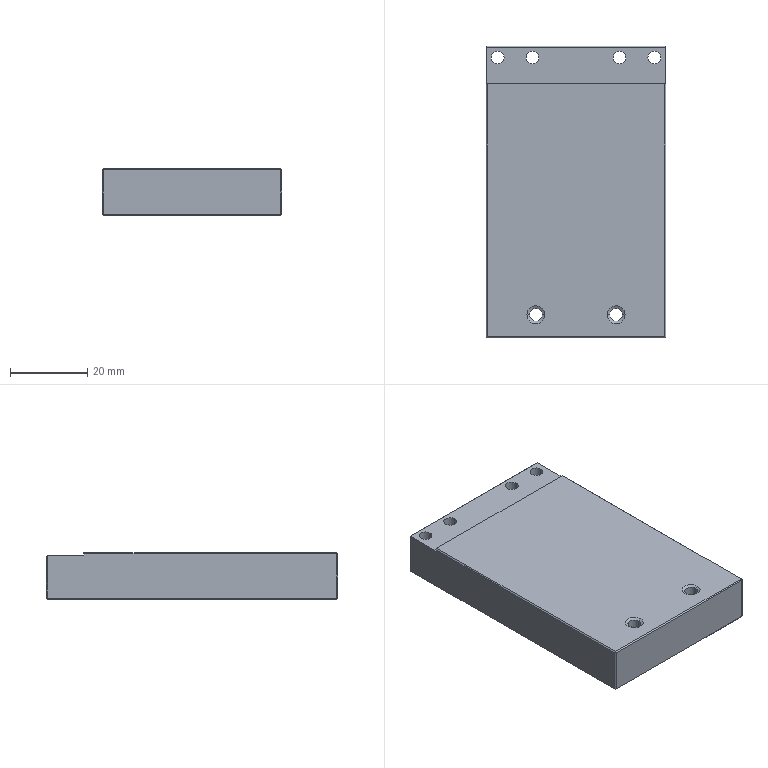Part | NX | 1 solid | 44 faces | box 46.5 x 75.4 x 12 mm | volume 41106 mm3 | plane 20 | cylinder 12 | cone 12 | commonest cylinder face diameters 3.3 x12
STEP:
#1=CARTESIAN_POINT('',(-134.2,260.1,-43.777));
#2=VERTEX_POINT('',#1);
#3=CARTESIAN_POINT('',(-88.3,260.1,-43.777));
#4=VERTEX_POINT('',#3);
#5=CARTESIAN_POINT('',(-111.25,260.1,-43.777));
#6=DIRECTION('',(1.,0.,0.));
#7=VECTOR('',#6,1000.);
#8=LINE('',#5,#7);
#9=EDGE_CURVE('',#2,#4,#8,.T.);
#10=ORIENTED_EDGE('',*,*,#9,.F.);
#11=CARTESIAN_POINT('',(-134.2,260.1,-33.14));
#12=VERTEX_POINT('',#11);
#13=CARTESIAN_POINT('',(-134.2,260.1,-38.458));
#14=DIRECTION('',(0.,0.,-1.));
#15=VECTOR('',#14,1000.);
#16=LINE('',#13,#15);
#17=EDGE_CURVE('',#12,#2,#16,.T.);
#18=ORIENTED_EDGE('',*,*,#17,.F.);
#19=CARTESIAN_POINT('',(-88.3,260.1,-33.14));
#20=VERTEX_POINT('',#19);
#21=CARTESIAN_POINT('',(-111.25,260.1,-33.14));
#22=DIRECTION('',(-1.,0.,0.));
#23=VECTOR('',#22,1000.);
#24=LINE('',#21,#23);
#25=EDGE_CURVE('',#20,#12,#24,.T.);
#26=ORIENTED_EDGE('',*,*,#25,.F.);
#27=CARTESIAN_POINT('',(-88.3,260.1,-38.458));
#28=DIRECTION('',(0.,0.,1.));
#29=VECTOR('',#28,1000.);
#30=LINE('',#27,#29);
#31=EDGE_CURVE('',#4,#20,#30,.T.);
#32=ORIENTED_EDGE('',*,*,#31,.F.);
#33=EDGE_LOOP('',(#10,#18,#26,#32));
#34=FACE_BOUND('',#33,.T.);
#35=CARTESIAN_POINT('',(-128.319,260.1,-42.779));
#36=DIRECTION('',(0.,1.,0.));
#37=DIRECTION('',(1.,0.,0.));
#38=AXIS2_PLACEMENT_3D('',#35,#36,#37);
#39=PLANE('',#38);
#40=ADVANCED_FACE('',(#34),#39,.T.);
#41=ORIENTED_EDGE('',*,*,#9,.T.);
#42=CARTESIAN_POINT('',(-88.15,259.95,-43.927));
#43=VERTEX_POINT('',#42);
#44=CARTESIAN_POINT('',(0.,171.8,-132.077));
#45=DIRECTION('',(0.5774,-0.5774,-0.5774));
#46=VECTOR('',#45,1000.);
#47=LINE('',#44,#46);
#48=EDGE_CURVE('',#4,#43,#47,.T.);
#49=ORIENTED_EDGE('',*,*,#48,.T.);
#50=CARTESIAN_POINT('',(-88.3,259.8,-44.077));
#51=VERTEX_POINT('',#50);
#52=CARTESIAN_POINT('',(0.,348.1,44.223));
#53=DIRECTION('',(-0.5774,-0.5774,-0.5774));
#54=VECTOR('',#53,1000.);
#55=LINE('',#52,#54);
#56=EDGE_CURVE('',#43,#51,#55,.T.);
#57=ORIENTED_EDGE('',*,*,#56,.T.);
#58=CARTESIAN_POINT('',(-134.2,259.8,-44.077));
#59=VERTEX_POINT('',#58);
#60=CARTESIAN_POINT('',(-111.25,259.8,-44.077));
#61=DIRECTION('',(1.,0.,0.));
#62=VECTOR('',#61,1000.);
#63=LINE('',#60,#62);
#64=EDGE_CURVE('',#59,#51,#63,.T.);
#65=ORIENTED_EDGE('',*,*,#64,.F.);
#66=CARTESIAN_POINT('',(-134.35,259.95,-43.927));
#67=VERTEX_POINT('',#66);
#68=CARTESIAN_POINT('',(125.6,0.,-303.877));
#69=DIRECTION('',(-0.5774,0.5774,0.5774));
#70=VECTOR('',#69,1000.);
#71=LINE('',#68,#70);
#72=EDGE_CURVE('',#59,#67,#71,.T.);
#73=ORIENTED_EDGE('',*,*,#72,.T.);
#74=CARTESIAN_POINT('',(0.,394.3,90.423));
#75=DIRECTION('',(-0.5774,-0.5774,-0.5774));
#76=VECTOR('',#75,1000.);
#77=LINE('',#74,#76);
#78=EDGE_CURVE('',#2,#67,#77,.T.);
#79=ORIENTED_EDGE('',*,*,#78,.F.);
#80=EDGE_LOOP('',(#41,#49,#57,#65,#73,#79));
#81=FACE_BOUND('',#80,.T.);
#82=CARTESIAN_POINT('',(-111.25,259.95,-43.927));
#83=DIRECTION('',(0.,-0.7071,0.7071));
#84=DIRECTION('',(-1.,0.,0.));
#85=AXIS2_PLACEMENT_3D('',#82,#83,#84);
#86=PLANE('',#85);
#87=ADVANCED_FACE('',(#81),#86,.F.);
#88=CARTESIAN_POINT('',(-134.5,185.,-32.377));
#89=VERTEX_POINT('',#88);
#90=CARTESIAN_POINT('',(-134.5,185.,-43.777));
#91=VERTEX_POINT('',#90);
#92=CARTESIAN_POINT('',(-134.5,185.,-37.927));
#93=DIRECTION('',(0.,0.,-1.));
#94=VECTOR('',#93,1000.);
#95=LINE('',#92,#94);
#96=EDGE_CURVE('',#89,#91,#95,.T.);
#97=ORIENTED_EDGE('',*,*,#96,.F.);
#98=CARTESIAN_POINT('',(-134.5,250.35,-32.377));
#99=VERTEX_POINT('',#98);
#100=CARTESIAN_POINT('',(-134.5,217.525,-32.377));
#101=DIRECTION('',(0.,1.,0.));
#102=VECTOR('',#101,1000.);
#103=LINE('',#100,#102);
#104=EDGE_CURVE('',#89,#99,#103,.T.);
#105=ORIENTED_EDGE('',*,*,#104,.T.);
#106=CARTESIAN_POINT('',(-134.5,250.35,-32.84));
#107=VERTEX_POINT('',#106);
#108=CARTESIAN_POINT('',(-134.5,250.35,0.));
#109=DIRECTION('',(0.,0.,1.));
#110=VECTOR('',#109,1000.);
#111=LINE('',#108,#110);
#112=EDGE_CURVE('',#107,#99,#111,.T.);
#113=ORIENTED_EDGE('',*,*,#112,.F.);
#114=CARTESIAN_POINT('',(-134.5,259.8,-32.84));
#115=VERTEX_POINT('',#114);
#116=CARTESIAN_POINT('',(-134.5,0.,-32.84));
#117=DIRECTION('',(0.,-1.,0.));
#118=VECTOR('',#117,1000.);
#119=LINE('',#116,#118);
#120=EDGE_CURVE('',#115,#107,#119,.T.);
#121=ORIENTED_EDGE('',*,*,#120,.F.);
#122=CARTESIAN_POINT('',(-134.5,259.8,-43.777));
#123=VERTEX_POINT('',#122);
#124=CARTESIAN_POINT('',(-134.5,259.8,-38.458));
#125=DIRECTION('',(0.,0.,-1.));
#126=VECTOR('',#125,1000.);
#127=LINE('',#124,#126);
#128=EDGE_CURVE('',#115,#123,#127,.T.);
#129=ORIENTED_EDGE('',*,*,#128,.T.);
#130=CARTESIAN_POINT('',(-134.5,222.55,-43.777));
#131=DIRECTION('',(0.,1.,0.));
#132=VECTOR('',#131,1000.);
#133=LINE('',#130,#132);
#134=EDGE_CURVE('',#91,#123,#133,.T.);
#135=ORIENTED_EDGE('',*,*,#134,.F.);
#136=EDGE_LOOP('',(#97,#105,#113,#121,#129,#135));
#137=FACE_BOUND('',#136,.T.);
#138=CARTESIAN_POINT('',(-134.5,208.7,-44.077));
#139=DIRECTION('',(-1.,0.,0.));
#140=DIRECTION('',(0.,0.,1.));
#141=AXIS2_PLACEMENT_3D('',#138,#139,#140);
#142=PLANE('',#141);
#143=ADVANCED_FACE('',(#137),#142,.T.);
#144=ORIENTED_EDGE('',*,*,#128,.F.);
#145=CARTESIAN_POINT('',(0.,394.3,-167.34));
#146=DIRECTION('',(-0.5774,-0.5774,0.5774));
#147=VECTOR('',#146,1000.);
#148=LINE('',#145,#147);
#149=EDGE_CURVE('',#12,#115,#148,.T.);
#150=ORIENTED_EDGE('',*,*,#149,.F.);
#151=ORIENTED_EDGE('',*,*,#17,.T.);
#152=ORIENTED_EDGE('',*,*,#78,.T.);
#153=CARTESIAN_POINT('',(-178.277,216.023,0.));
#154=DIRECTION('',(0.5774,0.5774,-0.5774));
#155=VECTOR('',#154,1000.);
#156=LINE('',#153,#155);
#157=EDGE_CURVE('',#123,#67,#156,.T.);
#158=ORIENTED_EDGE('',*,*,#157,.F.);
#159=EDGE_LOOP('',(#144,#150,#151,#152,#158));
#160=FACE_BOUND('',#159,.T.);
#161=CARTESIAN_POINT('',(-134.35,259.95,-38.458));
#162=DIRECTION('',(-0.7071,0.7071,0.));
#163=DIRECTION('',(0.,0.,1.));
#164=AXIS2_PLACEMENT_3D('',#161,#162,#163);
#165=PLANE('',#164);
#166=ADVANCED_FACE('',(#160),#165,.T.);
#167=ORIENTED_EDGE('',*,*,#134,.T.);
#168=ORIENTED_EDGE('',*,*,#157,.T.);
#169=ORIENTED_EDGE('',*,*,#72,.F.);
#170=CARTESIAN_POINT('',(-134.2,185.,-44.077));
#171=VERTEX_POINT('',#170);
#172=CARTESIAN_POINT('',(-134.2,222.55,-44.077));
#173=DIRECTION('',(0.,1.,0.));
#174=VECTOR('',#173,1000.);
#175=LINE('',#172,#174);
#176=EDGE_CURVE('',#171,#59,#175,.T.);
#177=ORIENTED_EDGE('',*,*,#176,.F.);
#178=CARTESIAN_POINT('',(-134.35,184.85,-43.927));
#179=VERTEX_POINT('',#178);
#180=CARTESIAN_POINT('',(-178.277,140.923,0.));
#181=DIRECTION('',(-0.5774,-0.5774,0.5774));
#182=VECTOR('',#181,1000.);
#183=LINE('',#180,#182);
#184=EDGE_CURVE('',#171,#179,#183,.T.);
#185=ORIENTED_EDGE('',*,*,#184,.T.);
#186=CARTESIAN_POINT('',(-178.277,228.777,0.));
#187=DIRECTION('',(0.5774,-0.5774,-0.5774));
#188=VECTOR('',#187,1000.);
#189=LINE('',#186,#188);
#190=EDGE_CURVE('',#91,#179,#189,.T.);
#191=ORIENTED_EDGE('',*,*,#190,.F.);
#192=EDGE_LOOP('',(#167,#168,#169,#177,#185,#191));
#193=FACE_BOUND('',#192,.T.);
#194=CARTESIAN_POINT('',(-134.35,222.55,-43.927));
#195=DIRECTION('',(0.7071,0.,0.7071));
#196=DIRECTION('',(0.,-1.,0.));
#197=AXIS2_PLACEMENT_3D('',#194,#195,#196);
#198=PLANE('',#197);
#199=ADVANCED_FACE('',(#193),#198,.F.);
#200=ORIENTED_EDGE('',*,*,#104,.F.);
#201=CARTESIAN_POINT('',(-134.35,184.85,-32.227));
#202=VERTEX_POINT('',#201);
#203=CARTESIAN_POINT('',(0.,50.5,102.123));
#204=DIRECTION('',(-0.5774,0.5774,-0.5774));
#205=VECTOR('',#204,1000.);
#206=LINE('',#203,#205);
#207=EDGE_CURVE('',#202,#89,#206,.T.);
#208=ORIENTED_EDGE('',*,*,#207,.F.);
#209=CARTESIAN_POINT('',(-134.2,185.,-32.077));
#210=VERTEX_POINT('',#209);
#211=CARTESIAN_POINT('',(0.,319.2,102.123));
#212=DIRECTION('',(-0.5774,-0.5774,-0.5774));
#213=VECTOR('',#212,1000.);
#214=LINE('',#211,#213);
#215=EDGE_CURVE('',#210,#202,#214,.T.);
#216=ORIENTED_EDGE('',*,*,#215,.F.);
#217=CARTESIAN_POINT('',(-134.2,250.35,-32.077));
#218=VERTEX_POINT('',#217);
#219=CARTESIAN_POINT('',(-134.2,217.525,-32.077));
#220=DIRECTION('',(0.,1.,0.));
#221=VECTOR('',#220,1000.);
#222=LINE('',#219,#221);
#223=EDGE_CURVE('',#210,#218,#222,.T.);
#224=ORIENTED_EDGE('',*,*,#223,.T.);
#225=CARTESIAN_POINT('',(0.,250.35,102.123));
#226=DIRECTION('',(0.7071,0.,0.7071));
#227=VECTOR('',#226,1000.);
#228=LINE('',#225,#227);
#229=EDGE_CURVE('',#99,#218,#228,.T.);
#230=ORIENTED_EDGE('',*,*,#229,.F.);
#231=EDGE_LOOP('',(#200,#208,#216,#224,#230));
#232=FACE_BOUND('',#231,.T.);
#233=CARTESIAN_POINT('',(-134.35,217.525,-32.227));
#234=DIRECTION('',(-0.7071,0.,0.7071));
#235=DIRECTION('',(0.,1.,0.));
#236=AXIS2_PLACEMENT_3D('',#233,#234,#235);
#237=PLANE('',#236);
#238=ADVANCED_FACE('',(#232),#237,.T.);
#239=ORIENTED_EDGE('',*,*,#96,.T.);
#240=ORIENTED_EDGE('',*,*,#190,.T.);
#241=CARTESIAN_POINT('',(-134.2,184.7,-43.777));
#242=VERTEX_POINT('',#241);
#243=CARTESIAN_POINT('',(50.5,0.,140.923));
#244=DIRECTION('',(0.5774,-0.5774,0.5774));
#245=VECTOR('',#244,1000.);
#246=LINE('',#243,#245);
#247=EDGE_CURVE('',#179,#242,#246,.T.);
#248=ORIENTED_EDGE('',*,*,#247,.T.);
#249=CARTESIAN_POINT('',(-134.2,184.7,-32.377));
#250=VERTEX_POINT('',#249);
#251=CARTESIAN_POINT('',(-134.2,184.7,-37.927));
#252=DIRECTION('',(0.,0.,-1.));
#253=VECTOR('',#252,1000.);
#254=LINE('',#251,#253);
#255=EDGE_CURVE('',#250,#242,#254,.T.);
#256=ORIENTED_EDGE('',*,*,#255,.F.);
#257=CARTESIAN_POINT('',(50.5,0.,-217.077));
#258=DIRECTION('',(-0.5774,0.5774,0.5774));
#259=VECTOR('',#258,1000.);
#260=LINE('',#257,#259);
#261=EDGE_CURVE('',#250,#202,#260,.T.);
#262=ORIENTED_EDGE('',*,*,#261,.T.);
#263=ORIENTED_EDGE('',*,*,#207,.T.);
#264=EDGE_LOOP('',(#239,#240,#248,#256,#262,#263));
#265=FACE_BOUND('',#264,.T.);
#266=CARTESIAN_POINT('',(-134.35,184.85,-37.927));
#267=DIRECTION('',(0.7071,0.7071,0.));
#268=DIRECTION('',(0.,0.,-1.));
#269=AXIS2_PLACEMENT_3D('',#266,#267,#268);
#270=PLANE('',#269);
#271=ADVANCED_FACE('',(#265),#270,.F.);
#272=CARTESIAN_POINT('',(-88.,259.8,-43.777));
#273=VERTEX_POINT('',#272);
#274=CARTESIAN_POINT('',(-88.,259.8,-32.84));
#275=VERTEX_POINT('',#274);
#276=CARTESIAN_POINT('',(-88.,259.8,-38.458));
#277=DIRECTION('',(0.,0.,1.));
#278=VECTOR('',#277,1000.);
#279=LINE('',#276,#278);
#280=EDGE_CURVE('',#273,#275,#279,.T.);
#281=ORIENTED_EDGE('',*,*,#280,.T.);
#282=CARTESIAN_POINT('',(-88.,250.35,-32.84));
#283=VERTEX_POINT('',#282);
#284=CARTESIAN_POINT('',(-88.,0.,-32.84));
#285=DIRECTION('',(0.,1.,0.));
#286=VECTOR('',#285,1000.);
#287=LINE('',#284,#286);
#288=EDGE_CURVE('',#283,#275,#287,.T.);
#289=ORIENTED_EDGE('',*,*,#288,.F.);
#290=CARTESIAN_POINT('',(-88.,250.35,-32.377));
#291=VERTEX_POINT('',#290);
#292=CARTESIAN_POINT('',(-88.,250.35,0.));
#293=DIRECTION('',(0.,0.,-1.));
#294=VECTOR('',#293,1000.);
#295=LINE('',#292,#294);
#296=EDGE_CURVE('',#291,#283,#295,.T.);
#297=ORIENTED_EDGE('',*,*,#296,.F.);
#298=CARTESIAN_POINT('',(-88.,185.,-32.377));
#299=VERTEX_POINT('',#298);
#300=CARTESIAN_POINT('',(-88.,217.525,-32.377));
#301=DIRECTION('',(0.,1.,0.));
#302=VECTOR('',#301,1000.);
#303=LINE('',#300,#302);
#304=EDGE_CURVE('',#299,#291,#303,.T.);
#305=ORIENTED_EDGE('',*,*,#304,.F.);
#306=CARTESIAN_POINT('',(-88.,185.,-43.777));
#307=VERTEX_POINT('',#306);
#308=CARTESIAN_POINT('',(-88.,185.,-37.927));
#309=DIRECTION('',(0.,0.,1.));
#310=VECTOR('',#309,1000.);
#311=LINE('',#308,#310);
#312=EDGE_CURVE('',#307,#299,#311,.T.);
#313=ORIENTED_EDGE('',*,*,#312,.F.);
#314=CARTESIAN_POINT('',(-88.,222.55,-43.777));
#315=DIRECTION('',(0.,1.,0.));
#316=VECTOR('',#315,1000.);
#317=LINE('',#314,#316);
#318=EDGE_CURVE('',#307,#273,#317,.T.);
#319=ORIENTED_EDGE('',*,*,#318,.T.);
#320=EDGE_LOOP('',(#281,#289,#297,#305,#313,#319));
#321=FACE_BOUND('',#320,.T.);
#322=CARTESIAN_POINT('',(-88.,208.7,-40.863));
#323=DIRECTION('',(1.,0.,0.));
#324=DIRECTION('',(0.,-1.,0.));
#325=AXIS2_PLACEMENT_3D('',#322,#323,#324);
#326=PLANE('',#325);
#327=ADVANCED_FACE('',(#321),#326,.T.);
#328=ORIENTED_EDGE('',*,*,#312,.T.);
#329=CARTESIAN_POINT('',(-88.15,184.85,-32.227));
#330=VERTEX_POINT('',#329);
#331=CARTESIAN_POINT('',(-273.,0.,152.623));
#332=DIRECTION('',(-0.5774,-0.5774,0.5774));
#333=VECTOR('',#332,1000.);
#334=LINE('',#331,#333);
#335=EDGE_CURVE('',#299,#330,#334,.T.);
#336=ORIENTED_EDGE('',*,*,#335,.T.);
#337=CARTESIAN_POINT('',(-88.3,184.7,-32.377));
#338=VERTEX_POINT('',#337);
#339=CARTESIAN_POINT('',(-273.,0.,-217.077));
#340=DIRECTION('',(0.5774,0.5774,0.5774));
#341=VECTOR('',#340,1000.);
#342=LINE('',#339,#341);
#343=EDGE_CURVE('',#338,#330,#342,.T.);
#344=ORIENTED_EDGE('',*,*,#343,.F.);
#345=CARTESIAN_POINT('',(-88.3,184.7,-43.777));
#346=VERTEX_POINT('',#345);
#347=CARTESIAN_POINT('',(-88.3,184.7,-37.927));
#348=DIRECTION('',(0.,0.,1.));
#349=VECTOR('',#348,1000.);
#350=LINE('',#347,#349);
#351=EDGE_CURVE('',#346,#338,#350,.T.);
#352=ORIENTED_EDGE('',*,*,#351,.F.);
#353=CARTESIAN_POINT('',(-88.15,184.85,-43.927));
#354=VERTEX_POINT('',#353);
#355=CARTESIAN_POINT('',(-132.077,140.923,0.));
#356=DIRECTION('',(0.5774,0.5774,-0.5774));
#357=VECTOR('',#356,1000.);
#358=LINE('',#355,#357);
#359=EDGE_CURVE('',#346,#354,#358,.T.);
#360=ORIENTED_EDGE('',*,*,#359,.T.);
#361=CARTESIAN_POINT('',(0.,273.,44.223));
#362=DIRECTION('',(0.5774,0.5774,0.5774));
#363=VECTOR('',#362,1000.);
#364=LINE('',#361,#363);
#365=EDGE_CURVE('',#354,#307,#364,.T.);
#366=ORIENTED_EDGE('',*,*,#365,.T.);
#367=EDGE_LOOP('',(#328,#336,#344,#352,#360,#366));
#368=FACE_BOUND('',#367,.T.);
#369=CARTESIAN_POINT('',(-88.15,184.85,-37.927));
#370=DIRECTION('',(-0.7071,0.7071,0.));
#371=DIRECTION('',(0.,0.,1.));
#372=AXIS2_PLACEMENT_3D('',#369,#370,#371);
#373=PLANE('',#372);
#374=ADVANCED_FACE('',(#368),#373,.F.);
#375=ORIENTED_EDGE('',*,*,#304,.T.);
#376=CARTESIAN_POINT('',(-88.3,250.35,-32.077));
#377=VERTEX_POINT('',#376);
#378=CARTESIAN_POINT('',(-120.377,250.35,0.));
#379=DIRECTION('',(-0.7071,0.,0.7071));
#380=VECTOR('',#379,1000.);
#381=LINE('',#378,#380);
#382=EDGE_CURVE('',#291,#377,#381,.T.);
#383=ORIENTED_EDGE('',*,*,#382,.T.);
#384=CARTESIAN_POINT('',(-88.3,185.,-32.077));
#385=VERTEX_POINT('',#384);
#386=CARTESIAN_POINT('',(-88.3,217.525,-32.077));
#387=DIRECTION('',(0.,1.,0.));
#388=VECTOR('',#387,1000.);
#389=LINE('',#386,#388);
#390=EDGE_CURVE('',#385,#377,#389,.T.);
#391=ORIENTED_EDGE('',*,*,#390,.F.);
#392=CARTESIAN_POINT('',(96.7,0.,-217.077));
#393=DIRECTION('',(-0.5774,0.5774,0.5774));
#394=VECTOR('',#393,1000.);
#395=LINE('',#392,#394);
#396=EDGE_CURVE('',#330,#385,#395,.T.);
#397=ORIENTED_EDGE('',*,*,#396,.F.);
#398=ORIENTED_EDGE('',*,*,#335,.F.);
#399=EDGE_LOOP('',(#375,#383,#391,#397,#398));
#400=FACE_BOUND('',#399,.T.);
#401=CARTESIAN_POINT('',(-88.15,217.525,-32.227));
#402=DIRECTION('',(-0.7071,0.,-0.7071));
#403=DIRECTION('',(-0.7071,0.,0.7071));
#404=AXIS2_PLACEMENT_3D('',#401,#402,#403);
#405=PLANE('',#404);
#406=ADVANCED_FACE('',(#400),#405,.F.);
#407=ORIENTED_EDGE('',*,*,#318,.F.);
#408=ORIENTED_EDGE('',*,*,#365,.F.);
#409=CARTESIAN_POINT('',(-88.3,185.,-44.077));
#410=VERTEX_POINT('',#409);
#411=CARTESIAN_POINT('',(0.,96.7,44.223));
#412=DIRECTION('',(0.5774,-0.5774,0.5774));
#413=VECTOR('',#412,1000.);
#414=LINE('',#411,#413);
#415=EDGE_CURVE('',#410,#354,#414,.T.);
#416=ORIENTED_EDGE('',*,*,#415,.F.);
#417=CARTESIAN_POINT('',(-88.3,222.55,-44.077));
#418=DIRECTION('',(0.,1.,0.));
#419=VECTOR('',#418,1000.);
#420=LINE('',#417,#419);
#421=EDGE_CURVE('',#410,#51,#420,.T.);
#422=ORIENTED_EDGE('',*,*,#421,.T.);
#423=ORIENTED_EDGE('',*,*,#56,.F.);
#424=CARTESIAN_POINT('',(0.,171.8,44.223));
#425=DIRECTION('',(0.5774,-0.5774,0.5774));
#426=VECTOR('',#425,1000.);
#427=LINE('',#424,#426);
#428=EDGE_CURVE('',#43,#273,#427,.T.);
#429=ORIENTED_EDGE('',*,*,#428,.T.);
#430=EDGE_LOOP('',(#407,#408,#416,#422,#423,#429));
#431=FACE_BOUND('',#430,.T.);
#432=CARTESIAN_POINT('',(-88.15,222.55,-43.927));
#433=DIRECTION('',(0.7071,0.,-0.7071));
#434=DIRECTION('',(0.,-1.,0.));
#435=AXIS2_PLACEMENT_3D('',#432,#433,#434);
#436=PLANE('',#435);
#437=ADVANCED_FACE('',(#431),#436,.T.);
#438=ORIENTED_EDGE('',*,*,#280,.F.);
#439=ORIENTED_EDGE('',*,*,#428,.F.);
#440=ORIENTED_EDGE('',*,*,#48,.F.);
#441=ORIENTED_EDGE('',*,*,#31,.T.);
#442=CARTESIAN_POINT('',(0.,171.8,55.16));
#443=DIRECTION('',(0.5774,-0.5774,0.5774));
#444=VECTOR('',#443,1000.);
#445=LINE('',#442,#444);
#446=EDGE_CURVE('',#20,#275,#445,.T.);
#447=ORIENTED_EDGE('',*,*,#446,.T.);
#448=EDGE_LOOP('',(#438,#439,#440,#441,#447));
#449=FACE_BOUND('',#448,.T.);
#450=CARTESIAN_POINT('',(-88.15,259.95,-38.458));
#451=DIRECTION('',(0.7071,0.7071,0.));
#452=DIRECTION('',(0.,0.,-1.));
#453=AXIS2_PLACEMENT_3D('',#450,#451,#452);
#454=PLANE('',#453);
#455=ADVANCED_FACE('',(#449),#454,.T.);
#456=CARTESIAN_POINT('',(-132.,185.,-44.077));
#457=DIRECTION('',(-1.,0.,0.));
#458=VECTOR('',#457,1000.);
#459=LINE('',#456,#458);
#460=EDGE_CURVE('',#410,#171,#459,.T.);
#461=ORIENTED_EDGE('',*,*,#460,.F.);
#462=ORIENTED_EDGE('',*,*,#415,.T.);
#463=ORIENTED_EDGE('',*,*,#359,.F.);
#464=CARTESIAN_POINT('',(-132.,184.7,-43.777));
#465=DIRECTION('',(-1.,0.,0.));
#466=VECTOR('',#465,1000.);
#467=LINE('',#464,#466);
#468=EDGE_CURVE('',#346,#242,#467,.T.);
#469=ORIENTED_EDGE('',*,*,#468,.T.);
#470=ORIENTED_EDGE('',*,*,#247,.F.);
#471=ORIENTED_EDGE('',*,*,#184,.F.);
#472=EDGE_LOOP('',(#461,#462,#463,#469,#470,#471));
#473=FACE_BOUND('',#472,.T.);
#474=CARTESIAN_POINT('',(-111.25,184.85,-43.927));
#475=DIRECTION('',(0.,0.7071,0.7071));
#476=DIRECTION('',(1.,0.,0.));
#477=AXIS2_PLACEMENT_3D('',#474,#475,#476);
#478=PLANE('',#477);
#479=ADVANCED_FACE('',(#473),#478,.F.);
#480=CARTESIAN_POINT('',(-111.25,185.,-32.077));
#481=DIRECTION('',(-1.,0.,0.));
#482=VECTOR('',#481,1000.);
#483=LINE('',#480,#482);
#484=EDGE_CURVE('',#385,#210,#483,.T.);
#485=ORIENTED_EDGE('',*,*,#484,.F.);
#486=ORIENTED_EDGE('',*,*,#390,.T.);
#487=CARTESIAN_POINT('',(0.,250.35,-32.077));
#488=DIRECTION('',(1.,0.,0.));
#489=VECTOR('',#488,1000.);
#490=LINE('',#487,#489);
#491=EDGE_CURVE('',#218,#377,#490,.T.);
#492=ORIENTED_EDGE('',*,*,#491,.F.);
#493=ORIENTED_EDGE('',*,*,#223,.F.);
#494=EDGE_LOOP('',(#485,#486,#492,#493));
#495=FACE_BOUND('',#494,.T.);
#496=CARTESIAN_POINT('',(-103.19,190.7,-32.077));
#497=VERTEX_POINT('',#496);
#498=CARTESIAN_POINT('',(-98.56,190.7,-32.077));
#499=VERTEX_POINT('',#498);
#500=CARTESIAN_POINT('',(-100.875,190.7,-32.077));
#501=DIRECTION('',(0.,0.,1.));
#502=DIRECTION('',(1.,0.,0.));
#503=AXIS2_PLACEMENT_3D('',#500,#501,#502);
#504=CIRCLE('',#503,2.315);
#505=EDGE_CURVE('',#497,#499,#504,.T.);
#506=ORIENTED_EDGE('',*,*,#505,.F.);
#507=CARTESIAN_POINT('',(-100.875,190.7,-32.077));
#508=DIRECTION('',(0.,0.,1.));
#509=DIRECTION('',(1.,0.,0.));
#510=AXIS2_PLACEMENT_3D('',#507,#508,#509);
#511=CIRCLE('',#510,2.315);
#512=EDGE_CURVE('',#499,#497,#511,.T.);
#513=ORIENTED_EDGE('',*,*,#512,.F.);
#514=EDGE_LOOP('',(#506,#513));
#515=FACE_BOUND('',#514,.T.);
#516=CARTESIAN_POINT('',(-123.94,190.7,-32.077));
#517=VERTEX_POINT('',#516);
#518=CARTESIAN_POINT('',(-119.31,190.7,-32.077));
#519=VERTEX_POINT('',#518);
#520=CARTESIAN_POINT('',(-121.625,190.7,-32.077));
#521=DIRECTION('',(0.,0.,1.));
#522=DIRECTION('',(1.,0.,0.));
#523=AXIS2_PLACEMENT_3D('',#520,#521,#522);
#524=CIRCLE('',#523,2.315);
#525=EDGE_CURVE('',#517,#519,#524,.T.);
#526=ORIENTED_EDGE('',*,*,#525,.F.);
#527=CARTESIAN_POINT('',(-121.625,190.7,-32.077));
#528=DIRECTION('',(0.,0.,1.));
#529=DIRECTION('',(1.,0.,0.));
#530=AXIS2_PLACEMENT_3D('',#527,#528,#529);
#531=CIRCLE('',#530,2.315);
#532=EDGE_CURVE('',#519,#517,#531,.T.);
#533=ORIENTED_EDGE('',*,*,#532,.F.);
#534=EDGE_LOOP('',(#526,#533));
#535=FACE_BOUND('',#534,.T.);
#536=CARTESIAN_POINT('',(-137.,208.7,-32.077));
#537=DIRECTION('',(0.,0.,1.));
#538=DIRECTION('',(1.,0.,0.));
#539=AXIS2_PLACEMENT_3D('',#536,#537,#538);
#540=PLANE('',#539);
#541=ADVANCED_FACE('',(#495,#515,#535),#540,.T.);
#542=CARTESIAN_POINT('',(-111.25,184.7,-32.377));
#543=DIRECTION('',(-1.,0.,0.));
#544=VECTOR('',#543,1000.);
#545=LINE('',#542,#544);
#546=EDGE_CURVE('',#338,#250,#545,.T.);
#547=ORIENTED_EDGE('',*,*,#546,.T.);
#548=ORIENTED_EDGE('',*,*,#255,.T.);
#549=ORIENTED_EDGE('',*,*,#468,.F.);
#550=ORIENTED_EDGE('',*,*,#351,.T.);
#551=EDGE_LOOP('',(#547,#548,#549,#550));
#552=FACE_BOUND('',#551,.T.);
#553=CARTESIAN_POINT('',(-128.319,184.7,-42.779));
#554=DIRECTION('',(0.,1.,0.));
#555=DIRECTION('',(1.,0.,0.));
#556=AXIS2_PLACEMENT_3D('',#553,#554,#555);
#557=PLANE('',#556);
#558=ADVANCED_FACE('',(#552),#557,.F.);
#559=CARTESIAN_POINT('',(-102.525,190.7,-32.461));
#560=VERTEX_POINT('',#559);
#561=CARTESIAN_POINT('',(-99.225,190.7,-32.461));
#562=VERTEX_POINT('',#561);
#563=CARTESIAN_POINT('',(-100.875,190.7,-32.461));
#564=DIRECTION('',(0.,0.,1.));
#565=DIRECTION('',(1.,0.,0.));
#566=AXIS2_PLACEMENT_3D('',#563,#564,#565);
#567=CIRCLE('',#566,1.65);
#568=EDGE_CURVE('',#560,#562,#567,.T.);
#569=ORIENTED_EDGE('',*,*,#568,.T.);
#570=CARTESIAN_POINT('',(-99.225,190.7,-44.077));
#571=VERTEX_POINT('',#570);
#572=CARTESIAN_POINT('',(-99.225,190.7,-36.077));
#573=DIRECTION('',(0.,0.,1.));
#574=VECTOR('',#573,1000.);
#575=LINE('',#572,#574);
#576=EDGE_CURVE('',#571,#562,#575,.T.);
#577=ORIENTED_EDGE('',*,*,#576,.F.);
#578=CARTESIAN_POINT('',(-102.525,190.7,-44.077));
#579=VERTEX_POINT('',#578);
#580=CARTESIAN_POINT('',(-100.875,190.7,-44.077));
#581=DIRECTION('',(0.,0.,1.));
#582=DIRECTION('',(1.,0.,0.));
#583=AXIS2_PLACEMENT_3D('',#580,#581,#582);
#584=CIRCLE('',#583,1.65);
#585=EDGE_CURVE('',#579,#571,#584,.T.);
#586=ORIENTED_EDGE('',*,*,#585,.F.);
#587=CARTESIAN_POINT('',(-102.525,190.7,-36.077));
#588=DIRECTION('',(0.,0.,1.));
#589=VECTOR('',#588,1000.);
#590=LINE('',#587,#589);
#591=EDGE_CURVE('',#579,#560,#590,.T.);
#592=ORIENTED_EDGE('',*,*,#591,.T.);
#593=EDGE_LOOP('',(#569,#577,#586,#592));
#594=FACE_BOUND('',#593,.T.);
#595=CARTESIAN_POINT('',(-100.875,190.7,-36.077));
#596=DIRECTION('',(0.,0.,1.));
#597=DIRECTION('',(1.,0.,0.));
#598=AXIS2_PLACEMENT_3D('',#595,#596,#597);
#599=CYLINDRICAL_SURFACE('',#598,1.65);
#600=ADVANCED_FACE('',(#594),#599,.F.);
#601=CARTESIAN_POINT('',(-89.35,257.1,-43.693));
#602=VERTEX_POINT('',#601);
#603=CARTESIAN_POINT('',(-92.65,257.1,-43.693));
#604=VERTEX_POINT('',#603);
#605=CARTESIAN_POINT('',(-91.,257.1,-43.693));
#606=DIRECTION('',(0.,0.,-1.));
#607=DIRECTION('',(-1.,0.,0.));
#608=AXIS2_PLACEMENT_3D('',#605,#606,#607);
#609=CIRCLE('',#608,1.65);
#610=EDGE_CURVE('',#602,#604,#609,.T.);
#611=ORIENTED_EDGE('',*,*,#610,.F.);
#612=CARTESIAN_POINT('',(-88.685,257.1,-44.077));
#613=VERTEX_POINT('',#612);
#614=CARTESIAN_POINT('',(-89.35,257.1,-43.693));
#615=DIRECTION('',(0.866,0.,-0.5));
#616=VECTOR('',#615,1000.);
#617=LINE('',#614,#616);
#618=EDGE_CURVE('',#613,#602,#617,.F.);
#619=ORIENTED_EDGE('',*,*,#618,.F.);
#620=CARTESIAN_POINT('',(-93.315,257.1,-44.077));
#621=VERTEX_POINT('',#620);
#622=CARTESIAN_POINT('',(-91.,257.1,-44.077));
#623=DIRECTION('',(0.,0.,-1.));
#624=DIRECTION('',(-1.,0.,0.));
#625=AXIS2_PLACEMENT_3D('',#622,#623,#624);
#626=CIRCLE('',#625,2.315);
#627=EDGE_CURVE('',#613,#621,#626,.T.);
#628=ORIENTED_EDGE('',*,*,#627,.T.);
#629=CARTESIAN_POINT('',(-92.65,257.1,-43.693));
#630=DIRECTION('',(-0.866,0.,-0.5));
#631=VECTOR('',#630,1000.);
#632=LINE('',#629,#631);
#633=EDGE_CURVE('',#621,#604,#632,.F.);
#634=ORIENTED_EDGE('',*,*,#633,.T.);
#635=EDGE_LOOP('',(#611,#619,#628,#634));
#636=FACE_BOUND('',#635,.T.);
#637=CARTESIAN_POINT('',(-91.,257.1,-43.693));
#638=DIRECTION('',(0.,0.,-1.));
#639=DIRECTION('',(-1.,0.,0.));
#640=AXIS2_PLACEMENT_3D('',#637,#638,#639);
#641=CONICAL_SURFACE('',#640,1.65,1.047);
#642=ADVANCED_FACE('',(#636),#641,.F.);
#643=ORIENTED_EDGE('',*,*,#460,.T.);
#644=ORIENTED_EDGE('',*,*,#176,.T.);
#645=ORIENTED_EDGE('',*,*,#64,.T.);
#646=ORIENTED_EDGE('',*,*,#421,.F.);
#647=EDGE_LOOP('',(#643,#644,#645,#646));
#648=FACE_BOUND('',#647,.T.);
#649=CARTESIAN_POINT('',(-97.685,257.1,-44.077));
#650=VERTEX_POINT('',#649);
#651=CARTESIAN_POINT('',(-102.315,257.1,-44.077));
#652=VERTEX_POINT('',#651);
#653=CARTESIAN_POINT('',(-100.,257.1,-44.077));
#654=DIRECTION('',(0.,0.,-1.));
#655=DIRECTION('',(-1.,0.,0.));
#656=AXIS2_PLACEMENT_3D('',#653,#654,#655);
#657=CIRCLE('',#656,2.315);
#658=EDGE_CURVE('',#650,#652,#657,.T.);
#659=ORIENTED_EDGE('',*,*,#658,.F.);
#660=CARTESIAN_POINT('',(-100.,257.1,-44.077));
#661=DIRECTION('',(0.,0.,-1.));
#662=DIRECTION('',(-1.,0.,0.));
#663=AXIS2_PLACEMENT_3D('',#660,#661,#662);
#664=CIRCLE('',#663,2.315);
#665=EDGE_CURVE('',#652,#650,#664,.T.);
#666=ORIENTED_EDGE('',*,*,#665,.F.);
#667=EDGE_LOOP('',(#659,#666));
#668=FACE_BOUND('',#667,.T.);
#669=CARTESIAN_POINT('',(-129.185,257.1,-44.077));
#670=VERTEX_POINT('',#669);
#671=CARTESIAN_POINT('',(-133.815,257.1,-44.077));
#672=VERTEX_POINT('',#671);
#673=CARTESIAN_POINT('',(-131.5,257.1,-44.077));
#674=DIRECTION('',(0.,0.,-1.));
#675=DIRECTION('',(-1.,0.,0.));
#676=AXIS2_PLACEMENT_3D('',#673,#674,#675);
#677=CIRCLE('',#676,2.315);
#678=EDGE_CURVE('',#670,#672,#677,.T.);
#679=ORIENTED_EDGE('',*,*,#678,.F.);
#680=CARTESIAN_POINT('',(-131.5,257.1,-44.077));
#681=DIRECTION('',(0.,0.,-1.));
#682=DIRECTION('',(-1.,0.,0.));
#683=AXIS2_PLACEMENT_3D('',#680,#681,#682);
#684=CIRCLE('',#683,2.315);
#685=EDGE_CURVE('',#672,#670,#684,.T.);
#686=ORIENTED_EDGE('',*,*,#685,.F.);
#687=EDGE_LOOP('',(#679,#686));
#688=FACE_BOUND('',#687,.T.);
#689=ORIENTED_EDGE('',*,*,#627,.F.);
#690=CARTESIAN_POINT('',(-91.,257.1,-44.077));
#691=DIRECTION('',(0.,0.,-1.));
#692=DIRECTION('',(-1.,0.,0.));
#693=AXIS2_PLACEMENT_3D('',#690,#691,#692);
#694=CIRCLE('',#693,2.315);
#695=EDGE_CURVE('',#621,#613,#694,.T.);
#696=ORIENTED_EDGE('',*,*,#695,.F.);
#697=EDGE_LOOP('',(#689,#696));
#698=FACE_BOUND('',#697,.T.);
#699=CARTESIAN_POINT('',(-123.275,190.7,-44.077));
#700=VERTEX_POINT('',#699);
#701=CARTESIAN_POINT('',(-119.975,190.7,-44.077));
#702=VERTEX_POINT('',#701);
#703=CARTESIAN_POINT('',(-121.625,190.7,-44.077));
#704=DIRECTION('',(0.,0.,1.));
#705=DIRECTION('',(1.,0.,0.));
#706=AXIS2_PLACEMENT_3D('',#703,#704,#705);
#707=CIRCLE('',#706,1.65);
#708=EDGE_CURVE('',#700,#702,#707,.T.);
#709=ORIENTED_EDGE('',*,*,#708,.T.);
#710=CARTESIAN_POINT('',(-121.625,190.7,-44.077));
#711=DIRECTION('',(0.,0.,1.));
#712=DIRECTION('',(1.,0.,0.));
#713=AXIS2_PLACEMENT_3D('',#710,#711,#712);
#714=CIRCLE('',#713,1.65);
#715=EDGE_CURVE('',#702,#700,#714,.T.);
#716=ORIENTED_EDGE('',*,*,#715,.T.);
#717=EDGE_LOOP('',(#709,#716));
#718=FACE_BOUND('',#717,.T.);
#719=CARTESIAN_POINT('',(-120.185,257.1,-44.077));
#720=VERTEX_POINT('',#719);
#721=CARTESIAN_POINT('',(-124.815,257.1,-44.077));
#722=VERTEX_POINT('',#721);
#723=CARTESIAN_POINT('',(-122.5,257.1,-44.077));
#724=DIRECTION('',(0.,0.,-1.));
#725=DIRECTION('',(-1.,0.,0.));
#726=AXIS2_PLACEMENT_3D('',#723,#724,#725);
#727=CIRCLE('',#726,2.315);
#728=EDGE_CURVE('',#720,#722,#727,.T.);
#729=ORIENTED_EDGE('',*,*,#728,.F.);
#730=CARTESIAN_POINT('',(-122.5,257.1,-44.077));
#731=DIRECTION('',(0.,0.,-1.));
#732=DIRECTION('',(-1.,0.,0.));
#733=AXIS2_PLACEMENT_3D('',#730,#731,#732);
#734=CIRCLE('',#733,2.315);
#735=EDGE_CURVE('',#722,#720,#734,.T.);
#736=ORIENTED_EDGE('',*,*,#735,.F.);
#737=EDGE_LOOP('',(#729,#736));
#738=FACE_BOUND('',#737,.T.);
#739=ORIENTED_EDGE('',*,*,#585,.T.);
#740=CARTESIAN_POINT('',(-100.875,190.7,-44.077));
#741=DIRECTION('',(0.,0.,1.));
#742=DIRECTION('',(1.,0.,0.));
#743=AXIS2_PLACEMENT_3D('',#740,#741,#742);
#744=CIRCLE('',#743,1.65);
#745=EDGE_CURVE('',#571,#579,#744,.T.);
#746=ORIENTED_EDGE('',*,*,#745,.T.);
#747=EDGE_LOOP('',(#739,#746));
#748=FACE_BOUND('',#747,.T.);
#749=CARTESIAN_POINT('',(-88.698,210.445,-44.077));
#750=DIRECTION('',(0.,0.,-1.));
#751=DIRECTION('',(0.,-1.,0.));
#752=AXIS2_PLACEMENT_3D('',#749,#750,#751);
#753=PLANE('',#752);
#754=ADVANCED_FACE('',(#648,#668,#688,#698,#718,#738,#748),#753,.T.);
#755=CARTESIAN_POINT('',(-123.275,190.7,-32.461));
#756=VERTEX_POINT('',#755);
#757=CARTESIAN_POINT('',(-119.975,190.7,-32.461));
#758=VERTEX_POINT('',#757);
#759=CARTESIAN_POINT('',(-121.625,190.7,-32.461));
#760=DIRECTION('',(0.,0.,1.));
#761=DIRECTION('',(1.,0.,0.));
#762=AXIS2_PLACEMENT_3D('',#759,#760,#761);
#763=CIRCLE('',#762,1.65);
#764=EDGE_CURVE('',#756,#758,#763,.T.);
#765=ORIENTED_EDGE('',*,*,#764,.T.);
#766=CARTESIAN_POINT('',(-119.975,190.7,-36.077));
#767=DIRECTION('',(0.,0.,1.));
#768=VECTOR('',#767,1000.);
#769=LINE('',#766,#768);
#770=EDGE_CURVE('',#702,#758,#769,.T.);
#771=ORIENTED_EDGE('',*,*,#770,.F.);
#772=ORIENTED_EDGE('',*,*,#708,.F.);
#773=CARTESIAN_POINT('',(-123.275,190.7,-36.077));
#774=DIRECTION('',(0.,0.,1.));
#775=VECTOR('',#774,1000.);
#776=LINE('',#773,#775);
#777=EDGE_CURVE('',#700,#756,#776,.T.);
#778=ORIENTED_EDGE('',*,*,#777,.T.);
#779=EDGE_LOOP('',(#765,#771,#772,#778));
#780=FACE_BOUND('',#779,.T.);
#781=CARTESIAN_POINT('',(-121.625,190.7,-36.077));
#782=DIRECTION('',(0.,0.,1.));
#783=DIRECTION('',(1.,0.,0.));
#784=AXIS2_PLACEMENT_3D('',#781,#782,#783);
#785=CYLINDRICAL_SURFACE('',#784,1.65);
#786=ADVANCED_FACE('',(#780),#785,.F.);
#787=ORIENTED_EDGE('',*,*,#764,.F.);
#788=CARTESIAN_POINT('',(-123.275,190.7,-32.461));
#789=DIRECTION('',(-0.866,0.,0.5));
#790=VECTOR('',#789,1000.);
#791=LINE('',#788,#790);
#792=EDGE_CURVE('',#756,#517,#791,.T.);
#793=ORIENTED_EDGE('',*,*,#792,.T.);
#794=ORIENTED_EDGE('',*,*,#525,.T.);
#795=CARTESIAN_POINT('',(-119.975,190.7,-32.461));
#796=DIRECTION('',(0.866,0.,0.5));
#797=VECTOR('',#796,1000.);
#798=LINE('',#795,#797);
#799=EDGE_CURVE('',#758,#519,#798,.T.);
#800=ORIENTED_EDGE('',*,*,#799,.F.);
#801=EDGE_LOOP('',(#787,#793,#794,#800));
#802=FACE_BOUND('',#801,.T.);
#803=CARTESIAN_POINT('',(-121.625,190.7,-32.461));
#804=DIRECTION('',(0.,0.,1.));
#805=DIRECTION('',(1.,0.,0.));
#806=AXIS2_PLACEMENT_3D('',#803,#804,#805);
#807=CONICAL_SURFACE('',#806,1.65,1.047);
#808=ADVANCED_FACE('',(#802),#807,.F.);
#809=ORIENTED_EDGE('',*,*,#568,.F.);
#810=CARTESIAN_POINT('',(-102.525,190.7,-32.461));
#811=DIRECTION('',(-0.866,0.,0.5));
#812=VECTOR('',#811,1000.);
#813=LINE('',#810,#812);
#814=EDGE_CURVE('',#560,#497,#813,.T.);
#815=ORIENTED_EDGE('',*,*,#814,.T.);
#816=ORIENTED_EDGE('',*,*,#505,.T.);
#817=CARTESIAN_POINT('',(-99.225,190.7,-32.461));
#818=DIRECTION('',(0.866,0.,0.5));
#819=VECTOR('',#818,1000.);
#820=LINE('',#817,#819);
#821=EDGE_CURVE('',#562,#499,#820,.T.);
#822=ORIENTED_EDGE('',*,*,#821,.F.);
#823=EDGE_LOOP('',(#809,#815,#816,#822));
#824=FACE_BOUND('',#823,.T.);
#825=CARTESIAN_POINT('',(-100.875,190.7,-32.461));
#826=DIRECTION('',(0.,0.,1.));
#827=DIRECTION('',(1.,0.,0.));
#828=AXIS2_PLACEMENT_3D('',#825,#826,#827);
#829=CONICAL_SURFACE('',#828,1.65,1.047);
#830=ADVANCED_FACE('',(#824),#829,.F.);
#831=ORIENTED_EDGE('',*,*,#112,.T.);
#832=ORIENTED_EDGE('',*,*,#229,.T.);
#833=ORIENTED_EDGE('',*,*,#491,.T.);
#834=ORIENTED_EDGE('',*,*,#382,.F.);
#835=ORIENTED_EDGE('',*,*,#296,.T.);
#836=CARTESIAN_POINT('',(-83.35,250.35,-32.84));
#837=DIRECTION('',(-1.,0.,0.));
#838=VECTOR('',#837,1000.);
#839=LINE('',#836,#838);
#840=EDGE_CURVE('',#283,#107,#839,.T.);
#841=ORIENTED_EDGE('',*,*,#840,.T.);
#842=EDGE_LOOP('',(#831,#832,#833,#834,#835,#841));
#843=FACE_BOUND('',#842,.T.);
#844=CARTESIAN_POINT('',(-83.35,250.35,39.16));
#845=DIRECTION('',(0.,-1.,0.));
#846=DIRECTION('',(-1.,0.,0.));
#847=AXIS2_PLACEMENT_3D('',#844,#845,#846);
#848=PLANE('',#847);
#849=ADVANCED_FACE('',(#843),#848,.F.);
#850=CARTESIAN_POINT('',(-111.25,259.8,-32.84));
#851=DIRECTION('',(-1.,0.,0.));
#852=VECTOR('',#851,1000.);
#853=LINE('',#850,#852);
#854=EDGE_CURVE('',#275,#115,#853,.T.);
#855=ORIENTED_EDGE('',*,*,#854,.T.);
#856=ORIENTED_EDGE('',*,*,#120,.T.);
#857=ORIENTED_EDGE('',*,*,#840,.F.);
#858=ORIENTED_EDGE('',*,*,#288,.T.);
#859=EDGE_LOOP('',(#855,#856,#857,#858));
#860=FACE_BOUND('',#859,.T.);
#861=CARTESIAN_POINT('',(-98.35,257.1,-32.84));
#862=VERTEX_POINT('',#861);
#863=CARTESIAN_POINT('',(-101.65,257.1,-32.84));
#864=VERTEX_POINT('',#863);
#865=CARTESIAN_POINT('',(-100.,257.1,-32.84));
#866=DIRECTION('',(0.,0.,-1.));
#867=DIRECTION('',(-1.,0.,0.));
#868=AXIS2_PLACEMENT_3D('',#865,#866,#867);
#869=CIRCLE('',#868,1.65);
#870=EDGE_CURVE('',#862,#864,#869,.T.);
#871=ORIENTED_EDGE('',*,*,#870,.T.);
#872=CARTESIAN_POINT('',(-100.,257.1,-32.84));
#873=DIRECTION('',(0.,0.,-1.));
#874=DIRECTION('',(-1.,0.,0.));
#875=AXIS2_PLACEMENT_3D('',#872,#873,#874);
#876=CIRCLE('',#875,1.65);
#877=EDGE_CURVE('',#864,#862,#876,.T.);
#878=ORIENTED_EDGE('',*,*,#877,.T.);
#879=EDGE_LOOP('',(#871,#878));
#880=FACE_BOUND('',#879,.T.);
#881=CARTESIAN_POINT('',(-89.35,257.1,-32.84));
#882=VERTEX_POINT('',#881);
#883=CARTESIAN_POINT('',(-92.65,257.1,-32.84));
#884=VERTEX_POINT('',#883);
#885=CARTESIAN_POINT('',(-91.,257.1,-32.84));
#886=DIRECTION('',(0.,0.,-1.));
#887=DIRECTION('',(-1.,0.,0.));
#888=AXIS2_PLACEMENT_3D('',#885,#886,#887);
#889=CIRCLE('',#888,1.65);
#890=EDGE_CURVE('',#882,#884,#889,.T.);
#891=ORIENTED_EDGE('',*,*,#890,.T.);
#892=CARTESIAN_POINT('',(-91.,257.1,-32.84));
#893=DIRECTION('',(0.,0.,-1.));
#894=DIRECTION('',(-1.,0.,0.));
#895=AXIS2_PLACEMENT_3D('',#892,#893,#894);
#896=CIRCLE('',#895,1.65);
#897=EDGE_CURVE('',#884,#882,#896,.T.);
#898=ORIENTED_EDGE('',*,*,#897,.T.);
#899=EDGE_LOOP('',(#891,#898));
#900=FACE_BOUND('',#899,.T.);
#901=CARTESIAN_POINT('',(-129.85,257.1,-32.84));
#902=VERTEX_POINT('',#901);
#903=CARTESIAN_POINT('',(-133.15,257.1,-32.84));
#904=VERTEX_POINT('',#903);
#905=CARTESIAN_POINT('',(-131.5,257.1,-32.84));
#906=DIRECTION('',(0.,0.,-1.));
#907=DIRECTION('',(-1.,0.,0.));
#908=AXIS2_PLACEMENT_3D('',#905,#906,#907);
#909=CIRCLE('',#908,1.65);
#910=EDGE_CURVE('',#902,#904,#909,.T.);
#911=ORIENTED_EDGE('',*,*,#910,.T.);
#912=CARTESIAN_POINT('',(-131.5,257.1,-32.84));
#913=DIRECTION('',(0.,0.,-1.));
#914=DIRECTION('',(-1.,0.,0.));
#915=AXIS2_PLACEMENT_3D('',#912,#913,#914);
#916=CIRCLE('',#915,1.65);
#917=EDGE_CURVE('',#904,#902,#916,.T.);
#918=ORIENTED_EDGE('',*,*,#917,.T.);
#919=EDGE_LOOP('',(#911,#918));
#920=FACE_BOUND('',#919,.T.);
#921=CARTESIAN_POINT('',(-120.85,257.1,-32.84));
#922=VERTEX_POINT('',#921);
#923=CARTESIAN_POINT('',(-124.15,257.1,-32.84));
#924=VERTEX_POINT('',#923);
#925=CARTESIAN_POINT('',(-122.5,257.1,-32.84));
#926=DIRECTION('',(0.,0.,-1.));
#927=DIRECTION('',(-1.,0.,0.));
#928=AXIS2_PLACEMENT_3D('',#925,#926,#927);
#929=CIRCLE('',#928,1.65);
#930=EDGE_CURVE('',#922,#924,#929,.T.);
#931=ORIENTED_EDGE('',*,*,#930,.T.);
#932=CARTESIAN_POINT('',(-122.5,257.1,-32.84));
#933=DIRECTION('',(0.,0.,-1.));
#934=DIRECTION('',(-1.,0.,0.));
#935=AXIS2_PLACEMENT_3D('',#932,#933,#934);
#936=CIRCLE('',#935,1.65);
#937=EDGE_CURVE('',#924,#922,#936,.T.);
#938=ORIENTED_EDGE('',*,*,#937,.T.);
#939=EDGE_LOOP('',(#931,#938));
#940=FACE_BOUND('',#939,.T.);
#941=CARTESIAN_POINT('',(-83.35,250.35,-32.84));
#942=DIRECTION('',(0.,0.,-1.));
#943=DIRECTION('',(0.,-1.,0.));
#944=AXIS2_PLACEMENT_3D('',#941,#942,#943);
#945=PLANE('',#944);
#946=ADVANCED_FACE('',(#860,#880,#900,#920,#940),#945,.F.);
#947=CARTESIAN_POINT('',(-129.85,257.1,-43.693));
#948=VERTEX_POINT('',#947);
#949=CARTESIAN_POINT('',(-133.15,257.1,-43.693));
#950=VERTEX_POINT('',#949);
#951=CARTESIAN_POINT('',(-131.5,257.1,-43.693));
#952=DIRECTION('',(0.,0.,-1.));
#953=DIRECTION('',(-1.,0.,0.));
#954=AXIS2_PLACEMENT_3D('',#951,#952,#953);
#955=CIRCLE('',#954,1.65);
#956=EDGE_CURVE('',#948,#950,#955,.T.);
#957=ORIENTED_EDGE('',*,*,#956,.T.);
#958=CARTESIAN_POINT('',(-133.15,257.1,-44.077));
#959=DIRECTION('',(0.,0.,-1.));
#960=VECTOR('',#959,1000.);
#961=LINE('',#958,#960);
#962=EDGE_CURVE('',#950,#904,#961,.F.);
#963=ORIENTED_EDGE('',*,*,#962,.T.);
#964=ORIENTED_EDGE('',*,*,#910,.F.);
#965=CARTESIAN_POINT('',(-129.85,257.1,-44.077));
#966=DIRECTION('',(0.,0.,-1.));
#967=VECTOR('',#966,1000.);
#968=LINE('',#965,#967);
#969=EDGE_CURVE('',#948,#902,#968,.F.);
#970=ORIENTED_EDGE('',*,*,#969,.F.);
#971=EDGE_LOOP('',(#957,#963,#964,#970));
#972=FACE_BOUND('',#971,.T.);
#973=CARTESIAN_POINT('',(-131.5,257.1,-44.077));
#974=DIRECTION('',(0.,0.,-1.));
#975=DIRECTION('',(-1.,0.,0.));
#976=AXIS2_PLACEMENT_3D('',#973,#974,#975);
#977=CYLINDRICAL_SURFACE('',#976,1.65);
#978=ADVANCED_FACE('',(#972),#977,.F.);
#979=ORIENTED_EDGE('',*,*,#956,.F.);
#980=CARTESIAN_POINT('',(-129.85,257.1,-43.693));
#981=DIRECTION('',(0.866,0.,-0.5));
#982=VECTOR('',#981,1000.);
#983=LINE('',#980,#982);
#984=EDGE_CURVE('',#670,#948,#983,.F.);
#985=ORIENTED_EDGE('',*,*,#984,.F.);
#986=ORIENTED_EDGE('',*,*,#678,.T.);
#987=CARTESIAN_POINT('',(-133.15,257.1,-43.693));
#988=DIRECTION('',(-0.866,0.,-0.5));
#989=VECTOR('',#988,1000.);
#990=LINE('',#987,#989);
#991=EDGE_CURVE('',#672,#950,#990,.F.);
#992=ORIENTED_EDGE('',*,*,#991,.T.);
#993=EDGE_LOOP('',(#979,#985,#986,#992));
#994=FACE_BOUND('',#993,.T.);
#995=CARTESIAN_POINT('',(-131.5,257.1,-43.693));
#996=DIRECTION('',(0.,0.,-1.));
#997=DIRECTION('',(-1.,0.,0.));
#998=AXIS2_PLACEMENT_3D('',#995,#996,#997);
#999=CONICAL_SURFACE('',#998,1.65,1.047);
#1000=ADVANCED_FACE('',(#994),#999,.F.);
#1001=CARTESIAN_POINT('',(-120.85,257.1,-43.693));
#1002=VERTEX_POINT('',#1001);
#1003=CARTESIAN_POINT('',(-124.15,257.1,-43.693));
#1004=VERTEX_POINT('',#1003);
#1005=CARTESIAN_POINT('',(-122.5,257.1,-43.693));
#1006=DIRECTION('',(0.,0.,-1.));
#1007=DIRECTION('',(-1.,0.,0.));
#1008=AXIS2_PLACEMENT_3D('',#1005,#1006,#1007);
#1009=CIRCLE('',#1008,1.65);
#1010=EDGE_CURVE('',#1002,#1004,#1009,.T.);
#1011=ORIENTED_EDGE('',*,*,#1010,.T.);
#1012=CARTESIAN_POINT('',(-124.15,257.1,-44.077));
#1013=DIRECTION('',(0.,0.,-1.));
#1014=VECTOR('',#1013,1000.);
#1015=LINE('',#1012,#1014);
#1016=EDGE_CURVE('',#1004,#924,#1015,.F.);
#1017=ORIENTED_EDGE('',*,*,#1016,.T.);
#1018=ORIENTED_EDGE('',*,*,#930,.F.);
#1019=CARTESIAN_POINT('',(-120.85,257.1,-44.077));
#1020=DIRECTION('',(0.,0.,-1.));
#1021=VECTOR('',#1020,1000.);
#1022=LINE('',#1019,#1021);
#1023=EDGE_CURVE('',#1002,#922,#1022,.F.);
#1024=ORIENTED_EDGE('',*,*,#1023,.F.);
#1025=EDGE_LOOP('',(#1011,#1017,#1018,#1024));
#1026=FACE_BOUND('',#1025,.T.);
#1027=CARTESIAN_POINT('',(-122.5,257.1,-44.077));
#1028=DIRECTION('',(0.,0.,-1.));
#1029=DIRECTION('',(-1.,0.,0.));
#1030=AXIS2_PLACEMENT_3D('',#1027,#1028,#1029);
#1031=CYLINDRICAL_SURFACE('',#1030,1.65);
#1032=ADVANCED_FACE('',(#1026),#1031,.F.);
#1033=ORIENTED_EDGE('',*,*,#1010,.F.);
#1034=CARTESIAN_POINT('',(-120.85,257.1,-43.693));
#1035=DIRECTION('',(0.866,0.,-0.5));
#1036=VECTOR('',#1035,1000.);
#1037=LINE('',#1034,#1036);
#1038=EDGE_CURVE('',#720,#1002,#1037,.F.);
#1039=ORIENTED_EDGE('',*,*,#1038,.F.);
#1040=ORIENTED_EDGE('',*,*,#728,.T.);
#1041=CARTESIAN_POINT('',(-124.15,257.1,-43.693));
#1042=DIRECTION('',(-0.866,0.,-0.5));
#1043=VECTOR('',#1042,1000.);
#1044=LINE('',#1041,#1043);
#1045=EDGE_CURVE('',#722,#1004,#1044,.F.);
#1046=ORIENTED_EDGE('',*,*,#1045,.T.);
#1047=EDGE_LOOP('',(#1033,#1039,#1040,#1046));
#1048=FACE_BOUND('',#1047,.T.);
#1049=CARTESIAN_POINT('',(-122.5,257.1,-43.693));
#1050=DIRECTION('',(0.,0.,-1.));
#1051=DIRECTION('',(-1.,0.,0.));
#1052=AXIS2_PLACEMENT_3D('',#1049,#1050,#1051);
#1053=CONICAL_SURFACE('',#1052,1.65,1.047);
#1054=ADVANCED_FACE('',(#1048),#1053,.F.);
#1055=CARTESIAN_POINT('',(-98.35,257.1,-43.693));
#1056=VERTEX_POINT('',#1055);
#1057=CARTESIAN_POINT('',(-101.65,257.1,-43.693));
#1058=VERTEX_POINT('',#1057);
#1059=CARTESIAN_POINT('',(-100.,257.1,-43.693));
#1060=DIRECTION('',(0.,0.,-1.));
#1061=DIRECTION('',(-1.,0.,0.));
#1062=AXIS2_PLACEMENT_3D('',#1059,#1060,#1061);
#1063=CIRCLE('',#1062,1.65);
#1064=EDGE_CURVE('',#1056,#1058,#1063,.T.);
#1065=ORIENTED_EDGE('',*,*,#1064,.T.);
#1066=CARTESIAN_POINT('',(-101.65,257.1,-44.077));
#1067=DIRECTION('',(0.,0.,-1.));
#1068=VECTOR('',#1067,1000.);
#1069=LINE('',#1066,#1068);
#1070=EDGE_CURVE('',#1058,#864,#1069,.F.);
#1071=ORIENTED_EDGE('',*,*,#1070,.T.);
#1072=ORIENTED_EDGE('',*,*,#870,.F.);
#1073=CARTESIAN_POINT('',(-98.35,257.1,-44.077));
#1074=DIRECTION('',(0.,0.,-1.));
#1075=VECTOR('',#1074,1000.);
#1076=LINE('',#1073,#1075);
#1077=EDGE_CURVE('',#1056,#862,#1076,.F.);
#1078=ORIENTED_EDGE('',*,*,#1077,.F.);
#1079=EDGE_LOOP('',(#1065,#1071,#1072,#1078));
#1080=FACE_BOUND('',#1079,.T.);
#1081=CARTESIAN_POINT('',(-100.,257.1,-44.077));
#1082=DIRECTION('',(0.,0.,-1.));
#1083=DIRECTION('',(-1.,0.,0.));
#1084=AXIS2_PLACEMENT_3D('',#1081,#1082,#1083);
#1085=CYLINDRICAL_SURFACE('',#1084,1.65);
#1086=ADVANCED_FACE('',(#1080),#1085,.F.);
#1087=ORIENTED_EDGE('',*,*,#1064,.F.);
#1088=CARTESIAN_POINT('',(-98.35,257.1,-43.693));
#1089=DIRECTION('',(0.866,0.,-0.5));
#1090=VECTOR('',#1089,1000.);
#1091=LINE('',#1088,#1090);
#1092=EDGE_CURVE('',#650,#1056,#1091,.F.);
#1093=ORIENTED_EDGE('',*,*,#1092,.F.);
#1094=ORIENTED_EDGE('',*,*,#658,.T.);
#1095=CARTESIAN_POINT('',(-101.65,257.1,-43.693));
#1096=DIRECTION('',(-0.866,0.,-0.5));
#1097=VECTOR('',#1096,1000.);
#1098=LINE('',#1095,#1097);
#1099=EDGE_CURVE('',#652,#1058,#1098,.F.);
#1100=ORIENTED_EDGE('',*,*,#1099,.T.);
#1101=EDGE_LOOP('',(#1087,#1093,#1094,#1100));
#1102=FACE_BOUND('',#1101,.T.);
#1103=CARTESIAN_POINT('',(-100.,257.1,-43.693));
#1104=DIRECTION('',(0.,0.,-1.));
#1105=DIRECTION('',(-1.,0.,0.));
#1106=AXIS2_PLACEMENT_3D('',#1103,#1104,#1105);
#1107=CONICAL_SURFACE('',#1106,1.65,1.047);
#1108=ADVANCED_FACE('',(#1102),#1107,.F.);
#1109=ORIENTED_EDGE('',*,*,#610,.T.);
#1110=CARTESIAN_POINT('',(-92.65,257.1,-44.077));
#1111=DIRECTION('',(0.,0.,-1.));
#1112=VECTOR('',#1111,1000.);
#1113=LINE('',#1110,#1112);
#1114=EDGE_CURVE('',#604,#884,#1113,.F.);
#1115=ORIENTED_EDGE('',*,*,#1114,.T.);
#1116=ORIENTED_EDGE('',*,*,#890,.F.);
#1117=CARTESIAN_POINT('',(-89.35,257.1,-44.077));
#1118=DIRECTION('',(0.,0.,-1.));
#1119=VECTOR('',#1118,1000.);
#1120=LINE('',#1117,#1119);
#1121=EDGE_CURVE('',#602,#882,#1120,.F.);
#1122=ORIENTED_EDGE('',*,*,#1121,.F.);
#1123=EDGE_LOOP('',(#1109,#1115,#1116,#1122));
#1124=FACE_BOUND('',#1123,.T.);
#1125=CARTESIAN_POINT('',(-91.,257.1,-44.077));
#1126=DIRECTION('',(0.,0.,-1.));
#1127=DIRECTION('',(-1.,0.,0.));
#1128=AXIS2_PLACEMENT_3D('',#1125,#1126,#1127);
#1129=CYLINDRICAL_SURFACE('',#1128,1.65);
#1130=ADVANCED_FACE('',(#1124),#1129,.F.);
#1131=ORIENTED_EDGE('',*,*,#546,.F.);
#1132=ORIENTED_EDGE('',*,*,#343,.T.);
#1133=ORIENTED_EDGE('',*,*,#396,.T.);
#1134=ORIENTED_EDGE('',*,*,#484,.T.);
#1135=ORIENTED_EDGE('',*,*,#215,.T.);
#1136=ORIENTED_EDGE('',*,*,#261,.F.);
#1137=EDGE_LOOP('',(#1131,#1132,#1133,#1134,#1135,#1136));
#1138=FACE_BOUND('',#1137,.T.);
#1139=CARTESIAN_POINT('',(-111.25,184.85,-32.227));
#1140=DIRECTION('',(0.,-0.7071,0.7071));
#1141=DIRECTION('',(-1.,0.,0.));
#1142=AXIS2_PLACEMENT_3D('',#1139,#1140,#1141);
#1143=PLANE('',#1142);
#1144=ADVANCED_FACE('',(#1138),#1143,.T.);
#1145=ORIENTED_EDGE('',*,*,#854,.F.);
#1146=ORIENTED_EDGE('',*,*,#446,.F.);
#1147=ORIENTED_EDGE('',*,*,#25,.T.);
#1148=ORIENTED_EDGE('',*,*,#149,.T.);
#1149=EDGE_LOOP('',(#1145,#1146,#1147,#1148));
#1150=FACE_BOUND('',#1149,.T.);
#1151=CARTESIAN_POINT('',(-111.25,259.95,-32.99));
#1152=DIRECTION('',(0.,0.7071,0.7071));
#1153=DIRECTION('',(1.,0.,0.));
#1154=AXIS2_PLACEMENT_3D('',#1151,#1152,#1153);
#1155=PLANE('',#1154);
#1156=ADVANCED_FACE('',(#1150),#1155,.T.);
#1157=ORIENTED_EDGE('',*,*,#633,.F.);
#1158=ORIENTED_EDGE('',*,*,#695,.T.);
#1159=ORIENTED_EDGE('',*,*,#618,.T.);
#1160=CARTESIAN_POINT('',(-91.,257.1,-43.693));
#1161=DIRECTION('',(0.,0.,-1.));
#1162=DIRECTION('',(-1.,0.,0.));
#1163=AXIS2_PLACEMENT_3D('',#1160,#1161,#1162);
#1164=CIRCLE('',#1163,1.65);
#1165=EDGE_CURVE('',#604,#602,#1164,.T.);
#1166=ORIENTED_EDGE('',*,*,#1165,.F.);
#1167=EDGE_LOOP('',(#1157,#1158,#1159,#1166));
#1168=FACE_BOUND('',#1167,.T.);
#1169=CARTESIAN_POINT('',(-91.,257.1,-43.693));
#1170=DIRECTION('',(0.,0.,-1.));
#1171=DIRECTION('',(-1.,0.,0.));
#1172=AXIS2_PLACEMENT_3D('',#1169,#1170,#1171);
#1173=CONICAL_SURFACE('',#1172,1.65,1.047);
#1174=ADVANCED_FACE('',(#1168),#1173,.F.);
#1175=ORIENTED_EDGE('',*,*,#962,.F.);
#1176=CARTESIAN_POINT('',(-131.5,257.1,-43.693));
#1177=DIRECTION('',(0.,0.,-1.));
#1178=DIRECTION('',(-1.,0.,0.));
#1179=AXIS2_PLACEMENT_3D('',#1176,#1177,#1178);
#1180=CIRCLE('',#1179,1.65);
#1181=EDGE_CURVE('',#950,#948,#1180,.T.);
#1182=ORIENTED_EDGE('',*,*,#1181,.T.);
#1183=ORIENTED_EDGE('',*,*,#969,.T.);
#1184=ORIENTED_EDGE('',*,*,#917,.F.);
#1185=EDGE_LOOP('',(#1175,#1182,#1183,#1184));
#1186=FACE_BOUND('',#1185,.T.);
#1187=CARTESIAN_POINT('',(-131.5,257.1,-44.077));
#1188=DIRECTION('',(0.,0.,-1.));
#1189=DIRECTION('',(-1.,0.,0.));
#1190=AXIS2_PLACEMENT_3D('',#1187,#1188,#1189);
#1191=CYLINDRICAL_SURFACE('',#1190,1.65);
#1192=ADVANCED_FACE('',(#1186),#1191,.F.);
#1193=ORIENTED_EDGE('',*,*,#576,.T.);
#1194=CARTESIAN_POINT('',(-100.875,190.7,-32.461));
#1195=DIRECTION('',(0.,0.,1.));
#1196=DIRECTION('',(1.,0.,0.));
#1197=AXIS2_PLACEMENT_3D('',#1194,#1195,#1196);
#1198=CIRCLE('',#1197,1.65);
#1199=EDGE_CURVE('',#562,#560,#1198,.T.);
#1200=ORIENTED_EDGE('',*,*,#1199,.T.);
#1201=ORIENTED_EDGE('',*,*,#591,.F.);
#1202=ORIENTED_EDGE('',*,*,#745,.F.);
#1203=EDGE_LOOP('',(#1193,#1200,#1201,#1202));
#1204=FACE_BOUND('',#1203,.T.);
#1205=CARTESIAN_POINT('',(-100.875,190.7,-36.077));
#1206=DIRECTION('',(0.,0.,1.));
#1207=DIRECTION('',(1.,0.,0.));
#1208=AXIS2_PLACEMENT_3D('',#1205,#1206,#1207);
#1209=CYLINDRICAL_SURFACE('',#1208,1.65);
#1210=ADVANCED_FACE('',(#1204),#1209,.F.);
#1211=ORIENTED_EDGE('',*,*,#1070,.F.);
#1212=CARTESIAN_POINT('',(-100.,257.1,-43.693));
#1213=DIRECTION('',(0.,0.,-1.));
#1214=DIRECTION('',(-1.,0.,0.));
#1215=AXIS2_PLACEMENT_3D('',#1212,#1213,#1214);
#1216=CIRCLE('',#1215,1.65);
#1217=EDGE_CURVE('',#1058,#1056,#1216,.T.);
#1218=ORIENTED_EDGE('',*,*,#1217,.T.);
#1219=ORIENTED_EDGE('',*,*,#1077,.T.);
#1220=ORIENTED_EDGE('',*,*,#877,.F.);
#1221=EDGE_LOOP('',(#1211,#1218,#1219,#1220));
#1222=FACE_BOUND('',#1221,.T.);
#1223=CARTESIAN_POINT('',(-100.,257.1,-44.077));
#1224=DIRECTION('',(0.,0.,-1.));
#1225=DIRECTION('',(-1.,0.,0.));
#1226=AXIS2_PLACEMENT_3D('',#1223,#1224,#1225);
#1227=CYLINDRICAL_SURFACE('',#1226,1.65);
#1228=ADVANCED_FACE('',(#1222),#1227,.F.);
#1229=ORIENTED_EDGE('',*,*,#1114,.F.);
#1230=ORIENTED_EDGE('',*,*,#1165,.T.);
#1231=ORIENTED_EDGE('',*,*,#1121,.T.);
#1232=ORIENTED_EDGE('',*,*,#897,.F.);
#1233=EDGE_LOOP('',(#1229,#1230,#1231,#1232));
#1234=FACE_BOUND('',#1233,.T.);
#1235=CARTESIAN_POINT('',(-91.,257.1,-44.077));
#1236=DIRECTION('',(0.,0.,-1.));
#1237=DIRECTION('',(-1.,0.,0.));
#1238=AXIS2_PLACEMENT_3D('',#1235,#1236,#1237);
#1239=CYLINDRICAL_SURFACE('',#1238,1.65);
#1240=ADVANCED_FACE('',(#1234),#1239,.F.);
#1241=ORIENTED_EDGE('',*,*,#1099,.F.);
#1242=ORIENTED_EDGE('',*,*,#665,.T.);
#1243=ORIENTED_EDGE('',*,*,#1092,.T.);
#1244=ORIENTED_EDGE('',*,*,#1217,.F.);
#1245=EDGE_LOOP('',(#1241,#1242,#1243,#1244));
#1246=FACE_BOUND('',#1245,.T.);
#1247=CARTESIAN_POINT('',(-100.,257.1,-43.693));
#1248=DIRECTION('',(0.,0.,-1.));
#1249=DIRECTION('',(-1.,0.,0.));
#1250=AXIS2_PLACEMENT_3D('',#1247,#1248,#1249);
#1251=CONICAL_SURFACE('',#1250,1.65,1.047);
#1252=ADVANCED_FACE('',(#1246),#1251,.F.);
#1253=ORIENTED_EDGE('',*,*,#799,.T.);
#1254=ORIENTED_EDGE('',*,*,#532,.T.);
#1255=ORIENTED_EDGE('',*,*,#792,.F.);
#1256=CARTESIAN_POINT('',(-121.625,190.7,-32.461));
#1257=DIRECTION('',(0.,0.,1.));
#1258=DIRECTION('',(1.,0.,0.));
#1259=AXIS2_PLACEMENT_3D('',#1256,#1257,#1258);
#1260=CIRCLE('',#1259,1.65);
#1261=EDGE_CURVE('',#758,#756,#1260,.T.);
#1262=ORIENTED_EDGE('',*,*,#1261,.F.);
#1263=EDGE_LOOP('',(#1253,#1254,#1255,#1262));
#1264=FACE_BOUND('',#1263,.T.);
#1265=CARTESIAN_POINT('',(-121.625,190.7,-32.461));
#1266=DIRECTION('',(0.,0.,1.));
#1267=DIRECTION('',(1.,0.,0.));
#1268=AXIS2_PLACEMENT_3D('',#1265,#1266,#1267);
#1269=CONICAL_SURFACE('',#1268,1.65,1.047);
#1270=ADVANCED_FACE('',(#1264),#1269,.F.);
#1271=ORIENTED_EDGE('',*,*,#1016,.F.);
#1272=CARTESIAN_POINT('',(-122.5,257.1,-43.693));
#1273=DIRECTION('',(0.,0.,-1.));
#1274=DIRECTION('',(-1.,0.,0.));
#1275=AXIS2_PLACEMENT_3D('',#1272,#1273,#1274);
#1276=CIRCLE('',#1275,1.65);
#1277=EDGE_CURVE('',#1004,#1002,#1276,.T.);
#1278=ORIENTED_EDGE('',*,*,#1277,.T.);
#1279=ORIENTED_EDGE('',*,*,#1023,.T.);
#1280=ORIENTED_EDGE('',*,*,#937,.F.);
#1281=EDGE_LOOP('',(#1271,#1278,#1279,#1280));
#1282=FACE_BOUND('',#1281,.T.);
#1283=CARTESIAN_POINT('',(-122.5,257.1,-44.077));
#1284=DIRECTION('',(0.,0.,-1.));
#1285=DIRECTION('',(-1.,0.,0.));
#1286=AXIS2_PLACEMENT_3D('',#1283,#1284,#1285);
#1287=CYLINDRICAL_SURFACE('',#1286,1.65);
#1288=ADVANCED_FACE('',(#1282),#1287,.F.);
#1289=ORIENTED_EDGE('',*,*,#991,.F.);
#1290=ORIENTED_EDGE('',*,*,#685,.T.);
#1291=ORIENTED_EDGE('',*,*,#984,.T.);
#1292=ORIENTED_EDGE('',*,*,#1181,.F.);
#1293=EDGE_LOOP('',(#1289,#1290,#1291,#1292));
#1294=FACE_BOUND('',#1293,.T.);
#1295=CARTESIAN_POINT('',(-131.5,257.1,-43.693));
#1296=DIRECTION('',(0.,0.,-1.));
#1297=DIRECTION('',(-1.,0.,0.));
#1298=AXIS2_PLACEMENT_3D('',#1295,#1296,#1297);
#1299=CONICAL_SURFACE('',#1298,1.65,1.047);
#1300=ADVANCED_FACE('',(#1294),#1299,.F.);
#1301=ORIENTED_EDGE('',*,*,#821,.T.);
#1302=ORIENTED_EDGE('',*,*,#512,.T.);
#1303=ORIENTED_EDGE('',*,*,#814,.F.);
#1304=ORIENTED_EDGE('',*,*,#1199,.F.);
#1305=EDGE_LOOP('',(#1301,#1302,#1303,#1304));
#1306=FACE_BOUND('',#1305,.T.);
#1307=CARTESIAN_POINT('',(-100.875,190.7,-32.461));
#1308=DIRECTION('',(0.,0.,1.));
#1309=DIRECTION('',(1.,0.,0.));
#1310=AXIS2_PLACEMENT_3D('',#1307,#1308,#1309);
#1311=CONICAL_SURFACE('',#1310,1.65,1.047);
#1312=ADVANCED_FACE('',(#1306),#1311,.F.);
#1313=ORIENTED_EDGE('',*,*,#770,.T.);
#1314=ORIENTED_EDGE('',*,*,#1261,.T.);
#1315=ORIENTED_EDGE('',*,*,#777,.F.);
#1316=ORIENTED_EDGE('',*,*,#715,.F.);
#1317=EDGE_LOOP('',(#1313,#1314,#1315,#1316));
#1318=FACE_BOUND('',#1317,.T.);
#1319=CARTESIAN_POINT('',(-121.625,190.7,-36.077));
#1320=DIRECTION('',(0.,0.,1.));
#1321=DIRECTION('',(1.,0.,0.));
#1322=AXIS2_PLACEMENT_3D('',#1319,#1320,#1321);
#1323=CYLINDRICAL_SURFACE('',#1322,1.65);
#1324=ADVANCED_FACE('',(#1318),#1323,.F.);
#1325=ORIENTED_EDGE('',*,*,#1045,.F.);
#1326=ORIENTED_EDGE('',*,*,#735,.T.);
#1327=ORIENTED_EDGE('',*,*,#1038,.T.);
#1328=ORIENTED_EDGE('',*,*,#1277,.F.);
#1329=EDGE_LOOP('',(#1325,#1326,#1327,#1328));
#1330=FACE_BOUND('',#1329,.T.);
#1331=CARTESIAN_POINT('',(-122.5,257.1,-43.693));
#1332=DIRECTION('',(0.,0.,-1.));
#1333=DIRECTION('',(-1.,0.,0.));
#1334=AXIS2_PLACEMENT_3D('',#1331,#1332,#1333);
#1335=CONICAL_SURFACE('',#1334,1.65,1.047);
#1336=ADVANCED_FACE('',(#1330),#1335,.F.);
#1337=CLOSED_SHELL('',(#40,#87,#143,#166,#199,#238,#271,#327,#374,#406,#437,#455,#479,#541,#558,#600,#642,#754,#786,#808,#830,#849,#946,#978,#1000,#1032,#1054,#1086,#1108,#1130,#1144,#1156,#1174,#1192,#1210,#1228,#1240,#1252,#1270,#1288,#1300,#1312,#1324,#1336));
#1338=MANIFOLD_SOLID_BREP('',#1337);
#1339=(LENGTH_UNIT()NAMED_UNIT(*)SI_UNIT(.MILLI.,.METRE.));
#1340=UNCERTAINTY_MEASURE_WITH_UNIT(LENGTH_MEASURE(0.00001),#1339,'','');
#1341=(NAMED_UNIT(*)PLANE_ANGLE_UNIT()SI_UNIT($,.RADIAN.));
#1342=(NAMED_UNIT(*)SI_UNIT($,.STERADIAN.)SOLID_ANGLE_UNIT());
#1343=(GEOMETRIC_REPRESENTATION_CONTEXT(3)GLOBAL_UNCERTAINTY_ASSIGNED_CONTEXT((#1340))GLOBAL_UNIT_ASSIGNED_CONTEXT((#1339,#1341,#1342))REPRESENTATION_CONTEXT('',''));
#1344=ADVANCED_BREP_SHAPE_REPRESENTATION('',(#1338),#1343);